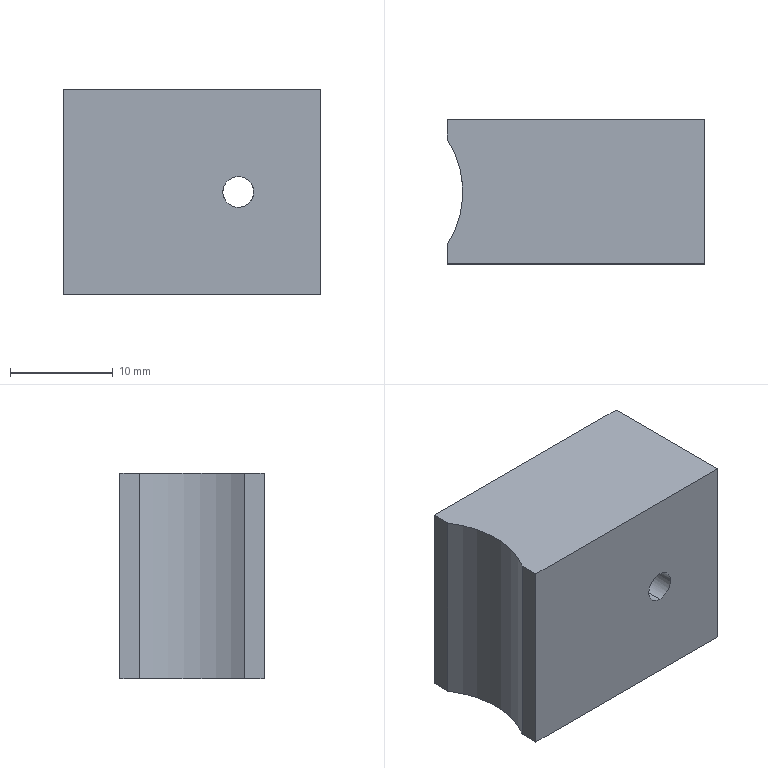Part | STEP file | push magnet block | 1 solid | 15 faces | box 25 x 14 x 20 mm | volume 5584 mm3 | plane 8 | cylinder 7 | commonest cylinder face diameters 3 x4 10 x2 19 x1